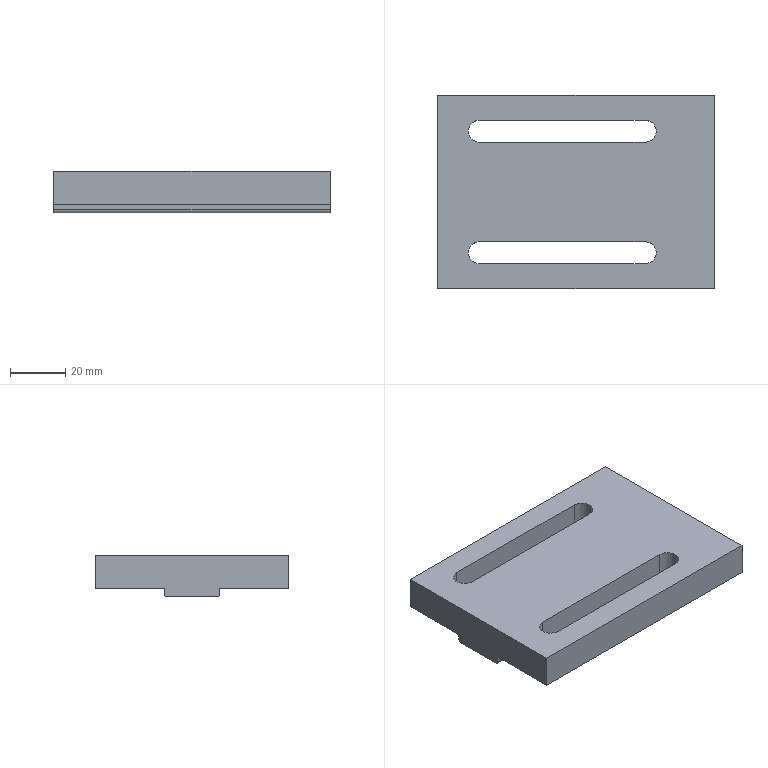Part | STEP file | Tube necking machine_id398_x_t | 1 solid | 20 faces | box 100 x 70 x 15 mm | volume 77231 mm3 | plane 14 | cylinder 6 | commonest cylinder face diameters 8 x4 2 x2